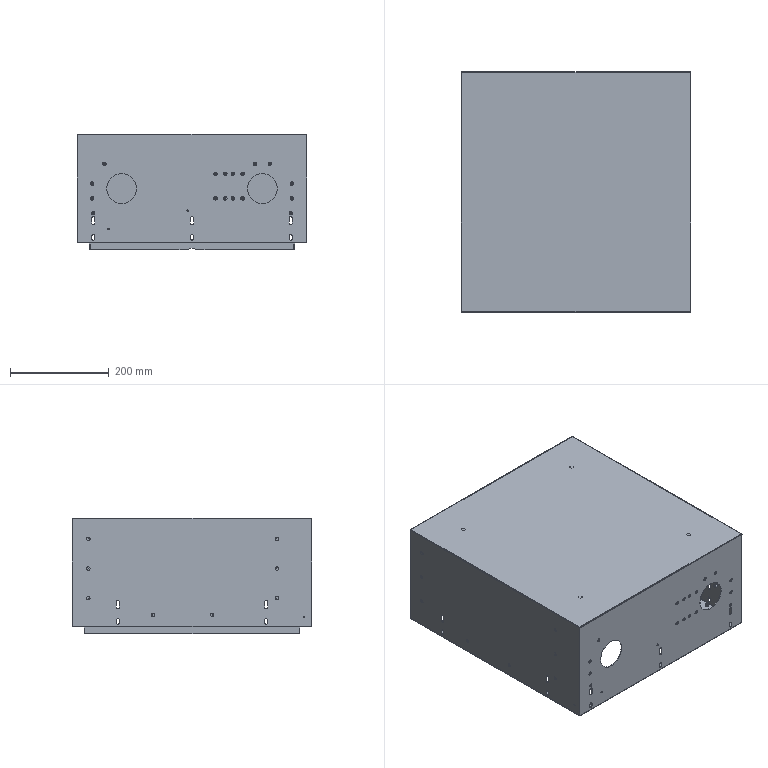Part | STEP file | 1 solid | 527 faces | box 465 x 486 x 234 mm | volume 846762 mm3 | cylinder 264 | plane 219 | cone 40 | spline 4 | commonest cylinder face diameters 7 x74 3.3 x70 6.2 x60 2.5 x16 0.02 x12 2.42 x12